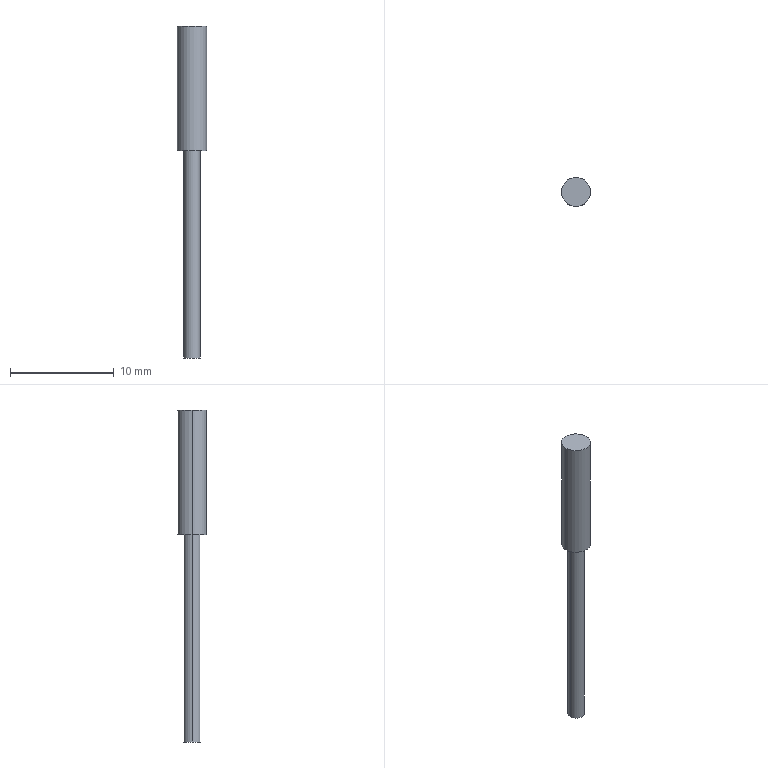Part | SolidWorks | features Extrusion 1, ICE 1 | 1 solid | 7 faces | box 2.8 x 2.8 x 32 mm | volume 114.103 mm3 | cylinder 4 | plane 3 | commonest cylinder face diameters 1.6 x2 2.8 x2
STEP:
#1=CARTESIAN_POINT('',(-0.8,0.,-20.));
#2=VERTEX_POINT('',#1);
#3=CARTESIAN_POINT('',(0.8,0.,-20.));
#4=VERTEX_POINT('',#3);
#5=CARTESIAN_POINT('',(0.,0.,-20.));
#6=DIRECTION('',(0.,0.,-1.));
#7=DIRECTION('',(-1.,0.,0.));
#8=AXIS2_PLACEMENT_3D('',#5,#6,#7);
#9=CIRCLE('',#8,0.8);
#10=EDGE_CURVE('',#2,#4,#9,.T.);
#11=ORIENTED_EDGE('',*,*,#10,.F.);
#12=CARTESIAN_POINT('',(-0.8,0.,0.));
#13=VERTEX_POINT('',#12);
#14=CARTESIAN_POINT('',(-0.8,0.,-20.));
#15=DIRECTION('',(0.,0.,1.));
#16=VECTOR('',#15,1000.);
#17=LINE('',#14,#16);
#18=EDGE_CURVE('',#2,#13,#17,.T.);
#19=ORIENTED_EDGE('',*,*,#18,.T.);
#20=CARTESIAN_POINT('',(0.8,0.,0.));
#21=VERTEX_POINT('',#20);
#22=CARTESIAN_POINT('',(0.,0.,0.));
#23=DIRECTION('',(0.,0.,-1.));
#24=DIRECTION('',(1.,0.,0.));
#25=AXIS2_PLACEMENT_3D('',#22,#23,#24);
#26=CIRCLE('',#25,0.8);
#27=EDGE_CURVE('',#13,#21,#26,.T.);
#28=ORIENTED_EDGE('',*,*,#27,.T.);
#29=CARTESIAN_POINT('',(0.8,0.,-20.));
#30=DIRECTION('',(0.,0.,1.));
#31=VECTOR('',#30,1000.);
#32=LINE('',#29,#31);
#33=EDGE_CURVE('',#4,#21,#32,.T.);
#34=ORIENTED_EDGE('',*,*,#33,.F.);
#35=EDGE_LOOP('',(#11,#19,#28,#34));
#36=FACE_OUTER_BOUND('',#35,.T.);
#37=CARTESIAN_POINT('',(0.,0.,-20.));
#38=DIRECTION('',(0.,0.,1.));
#39=DIRECTION('',(1.,0.,0.));
#40=AXIS2_PLACEMENT_3D('',#37,#38,#39);
#41=CYLINDRICAL_SURFACE('',#40,0.8);
#42=ADVANCED_FACE('',(#36),#41,.T.);
#43=CARTESIAN_POINT('',(1.4,0.,12.));
#44=VERTEX_POINT('',#43);
#45=CARTESIAN_POINT('',(-1.4,0.,12.));
#46=VERTEX_POINT('',#45);
#47=CARTESIAN_POINT('',(0.,0.,12.));
#48=DIRECTION('',(0.,0.,1.));
#49=DIRECTION('',(1.,0.,0.));
#50=AXIS2_PLACEMENT_3D('',#47,#48,#49);
#51=CIRCLE('',#50,1.4);
#52=EDGE_CURVE('',#44,#46,#51,.T.);
#53=ORIENTED_EDGE('',*,*,#52,.F.);
#54=CARTESIAN_POINT('',(1.4,0.,0.));
#55=VERTEX_POINT('',#54);
#56=CARTESIAN_POINT('',(1.4,0.,12.));
#57=DIRECTION('',(0.,0.,-1.));
#58=VECTOR('',#57,1000.);
#59=LINE('',#56,#58);
#60=EDGE_CURVE('',#44,#55,#59,.T.);
#61=ORIENTED_EDGE('',*,*,#60,.T.);
#62=CARTESIAN_POINT('',(-1.4,0.,0.));
#63=VERTEX_POINT('',#62);
#64=CARTESIAN_POINT('',(0.,0.,0.));
#65=DIRECTION('',(0.,0.,1.));
#66=DIRECTION('',(1.,0.,0.));
#67=AXIS2_PLACEMENT_3D('',#64,#65,#66);
#68=CIRCLE('',#67,1.4);
#69=EDGE_CURVE('',#55,#63,#68,.T.);
#70=ORIENTED_EDGE('',*,*,#69,.T.);
#71=CARTESIAN_POINT('',(-1.4,0.,12.));
#72=DIRECTION('',(0.,0.,-1.));
#73=VECTOR('',#72,1000.);
#74=LINE('',#71,#73);
#75=EDGE_CURVE('',#46,#63,#74,.T.);
#76=ORIENTED_EDGE('',*,*,#75,.F.);
#77=EDGE_LOOP('',(#53,#61,#70,#76));
#78=FACE_OUTER_BOUND('',#77,.T.);
#79=CARTESIAN_POINT('',(0.,0.,12.));
#80=DIRECTION('',(0.,0.,-1.));
#81=DIRECTION('',(-1.,0.,0.));
#82=AXIS2_PLACEMENT_3D('',#79,#80,#81);
#83=CYLINDRICAL_SURFACE('',#82,1.4);
#84=ADVANCED_FACE('',(#78),#83,.T.);
#85=CARTESIAN_POINT('',(0.,0.,0.));
#86=DIRECTION('',(0.,0.,1.));
#87=DIRECTION('',(1.,0.,0.));
#88=AXIS2_PLACEMENT_3D('',#85,#86,#87);
#89=CIRCLE('',#88,1.4);
#90=EDGE_CURVE('',#63,#55,#89,.T.);
#91=ORIENTED_EDGE('',*,*,#90,.F.);
#92=ORIENTED_EDGE('',*,*,#69,.F.);
#93=EDGE_LOOP('',(#91,#92));
#94=FACE_OUTER_BOUND('',#93,.T.);
#95=CARTESIAN_POINT('',(0.,0.,0.));
#96=DIRECTION('',(0.,0.,-1.));
#97=DIRECTION('',(1.,0.,0.));
#98=AXIS2_PLACEMENT_3D('',#95,#96,#97);
#99=CIRCLE('',#98,0.8);
#100=EDGE_CURVE('',#21,#13,#99,.T.);
#101=ORIENTED_EDGE('',*,*,#100,.F.);
#102=ORIENTED_EDGE('',*,*,#27,.F.);
#103=EDGE_LOOP('',(#101,#102));
#104=FACE_BOUND('',#103,.T.);
#105=CARTESIAN_POINT('',(0.,0.,0.));
#106=DIRECTION('',(0.,0.,1.));
#107=DIRECTION('',(1.,0.,0.));
#108=AXIS2_PLACEMENT_3D('',#105,#106,#107);
#109=PLANE('',#108);
#110=ADVANCED_FACE('',(#94,#104),#109,.F.);
#111=ORIENTED_EDGE('',*,*,#60,.F.);
#112=CARTESIAN_POINT('',(0.,0.,12.));
#113=DIRECTION('',(0.,0.,1.));
#114=DIRECTION('',(1.,0.,0.));
#115=AXIS2_PLACEMENT_3D('',#112,#113,#114);
#116=CIRCLE('',#115,1.4);
#117=EDGE_CURVE('',#46,#44,#116,.T.);
#118=ORIENTED_EDGE('',*,*,#117,.F.);
#119=ORIENTED_EDGE('',*,*,#75,.T.);
#120=ORIENTED_EDGE('',*,*,#90,.T.);
#121=EDGE_LOOP('',(#111,#118,#119,#120));
#122=FACE_OUTER_BOUND('',#121,.T.);
#123=CARTESIAN_POINT('',(0.,0.,12.));
#124=DIRECTION('',(0.,0.,-1.));
#125=DIRECTION('',(-1.,0.,0.));
#126=AXIS2_PLACEMENT_3D('',#123,#124,#125);
#127=CYLINDRICAL_SURFACE('',#126,1.4);
#128=ADVANCED_FACE('',(#122),#127,.T.);
#129=ORIENTED_EDGE('',*,*,#117,.T.);
#130=ORIENTED_EDGE('',*,*,#52,.T.);
#131=EDGE_LOOP('',(#129,#130));
#132=FACE_OUTER_BOUND('',#131,.T.);
#133=CARTESIAN_POINT('',(0.,0.,12.));
#134=DIRECTION('',(0.,0.,1.));
#135=DIRECTION('',(1.,0.,0.));
#136=AXIS2_PLACEMENT_3D('',#133,#134,#135);
#137=PLANE('',#136);
#138=ADVANCED_FACE('',(#132),#137,.T.);
#139=ORIENTED_EDGE('',*,*,#18,.F.);
#140=CARTESIAN_POINT('',(0.,0.,-20.));
#141=DIRECTION('',(0.,0.,-1.));
#142=DIRECTION('',(-1.,0.,0.));
#143=AXIS2_PLACEMENT_3D('',#140,#141,#142);
#144=CIRCLE('',#143,0.8);
#145=EDGE_CURVE('',#4,#2,#144,.T.);
#146=ORIENTED_EDGE('',*,*,#145,.F.);
#147=ORIENTED_EDGE('',*,*,#33,.T.);
#148=ORIENTED_EDGE('',*,*,#100,.T.);
#149=EDGE_LOOP('',(#139,#146,#147,#148));
#150=FACE_OUTER_BOUND('',#149,.T.);
#151=CARTESIAN_POINT('',(0.,0.,-20.));
#152=DIRECTION('',(0.,0.,1.));
#153=DIRECTION('',(1.,0.,0.));
#154=AXIS2_PLACEMENT_3D('',#151,#152,#153);
#155=CYLINDRICAL_SURFACE('',#154,0.8);
#156=ADVANCED_FACE('',(#150),#155,.T.);
#157=ORIENTED_EDGE('',*,*,#145,.T.);
#158=ORIENTED_EDGE('',*,*,#10,.T.);
#159=EDGE_LOOP('',(#157,#158));
#160=FACE_OUTER_BOUND('',#159,.T.);
#161=CARTESIAN_POINT('',(0.,0.,-20.));
#162=DIRECTION('',(0.,0.,-1.));
#163=DIRECTION('',(-1.,0.,0.));
#164=AXIS2_PLACEMENT_3D('',#161,#162,#163);
#165=PLANE('',#164);
#166=ADVANCED_FACE('',(#160),#165,.T.);
#167=CLOSED_SHELL('',(#42,#84,#110,#128,#138,#156,#166));
#168=MANIFOLD_SOLID_BREP('',#167);
#169=CARTESIAN_POINT('',(0.,0.,0.));
#170=DIRECTION('',(0.,0.,1.));
#171=DIRECTION('',(1.,0.,0.));
#172=AXIS2_PLACEMENT_3D('',#169,#170,#171);
#173=(LENGTH_UNIT()NAMED_UNIT(*)SI_UNIT(.MILLI.,.METRE.));
#174=UNCERTAINTY_MEASURE_WITH_UNIT(LENGTH_MEASURE(0.00001),#173,'','');
#175=(NAMED_UNIT(*)PLANE_ANGLE_UNIT()SI_UNIT($,.RADIAN.));
#176=(NAMED_UNIT(*)SI_UNIT($,.STERADIAN.)SOLID_ANGLE_UNIT());
#177=(GEOMETRIC_REPRESENTATION_CONTEXT(3)GLOBAL_UNCERTAINTY_ASSIGNED_CONTEXT((#174))GLOBAL_UNIT_ASSIGNED_CONTEXT((#173,#175,#176))REPRESENTATION_CONTEXT('',''));
#178=ADVANCED_BREP_SHAPE_REPRESENTATION('',(#168,#172),#177);